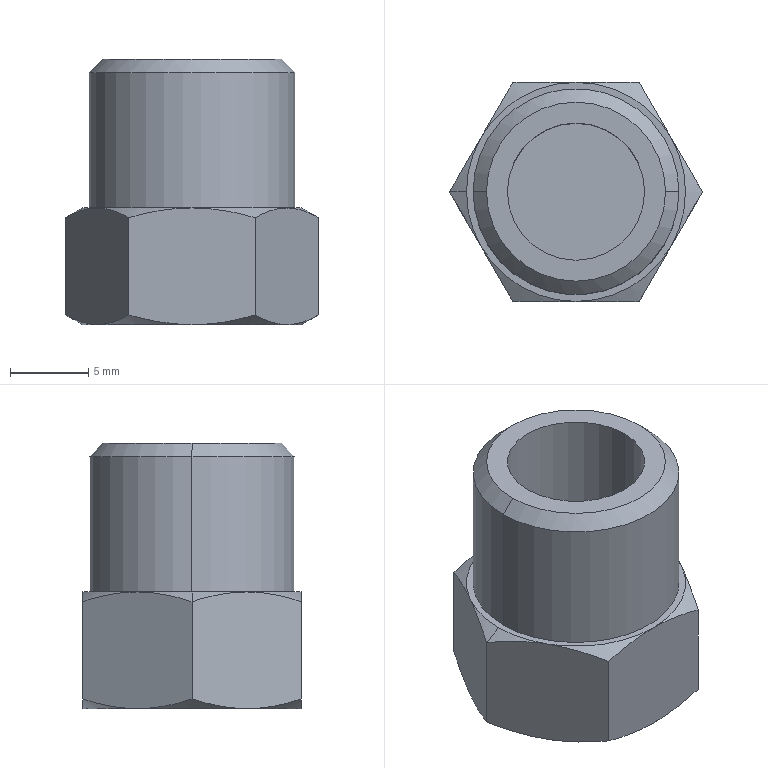Part | STEP file | Silencer BSLM02_APC6-02 | 1 solid | 33 faces | box 16.166 x 14 x 16.962 mm | volume 1893 mm3 | cone 16 | plane 11 | cylinder 6 | commonest cylinder face diameters 8.771 x2 11.5 x2 13.157 x2